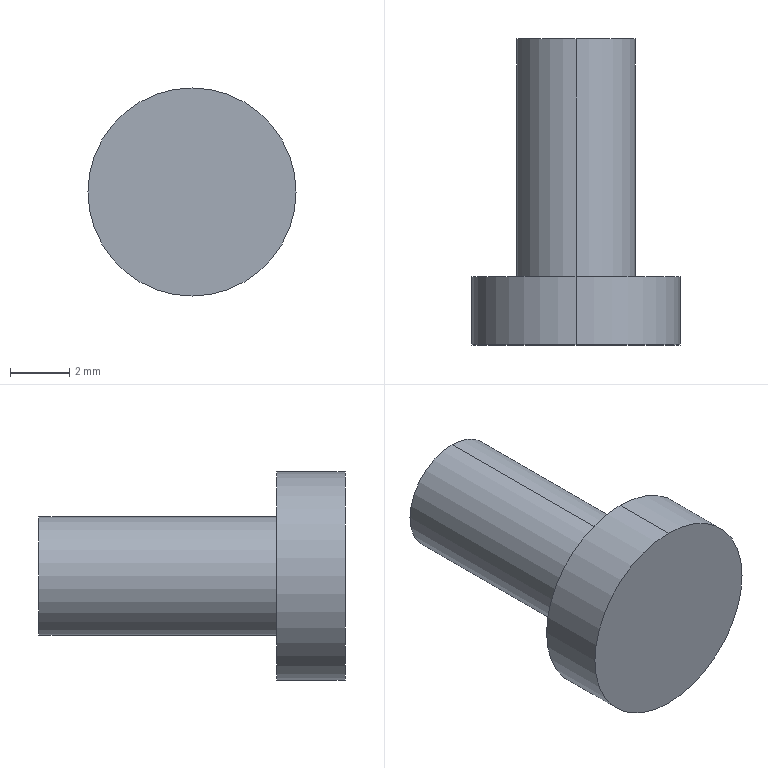Part | SolidWorks | features Extrusion 1, ICE 1 | 1 solid | 7 faces | box 7 x 10.3 x 7 mm | volume 189.045 mm3 | cylinder 4 | plane 3 | commonest cylinder face diameters 4 x2 7 x2
STEP:
#1=CARTESIAN_POINT('',(0.,-2.3,-3.5));
#2=VERTEX_POINT('',#1);
#3=CARTESIAN_POINT('',(0.,-2.3,3.5));
#4=VERTEX_POINT('',#3);
#5=CARTESIAN_POINT('',(0.,-2.3,0.));
#6=DIRECTION('',(0.,-1.,0.));
#7=DIRECTION('',(0.,0.,-1.));
#8=AXIS2_PLACEMENT_3D('',#5,#6,#7);
#9=CIRCLE('',#8,3.5);
#10=EDGE_CURVE('',#2,#4,#9,.T.);
#11=ORIENTED_EDGE('',*,*,#10,.F.);
#12=CARTESIAN_POINT('',(0.,0.,-3.5));
#13=VERTEX_POINT('',#12);
#14=CARTESIAN_POINT('',(0.,-2.3,-3.5));
#15=DIRECTION('',(0.,1.,0.));
#16=VECTOR('',#15,1000.);
#17=LINE('',#14,#16);
#18=EDGE_CURVE('',#2,#13,#17,.T.);
#19=ORIENTED_EDGE('',*,*,#18,.T.);
#20=CARTESIAN_POINT('',(0.,0.,3.5));
#21=VERTEX_POINT('',#20);
#22=CARTESIAN_POINT('',(0.,0.,0.));
#23=DIRECTION('',(0.,-1.,0.));
#24=DIRECTION('',(0.,0.,-1.));
#25=AXIS2_PLACEMENT_3D('',#22,#23,#24);
#26=CIRCLE('',#25,3.5);
#27=EDGE_CURVE('',#13,#21,#26,.T.);
#28=ORIENTED_EDGE('',*,*,#27,.T.);
#29=CARTESIAN_POINT('',(0.,-2.3,3.5));
#30=DIRECTION('',(0.,1.,0.));
#31=VECTOR('',#30,1000.);
#32=LINE('',#29,#31);
#33=EDGE_CURVE('',#4,#21,#32,.T.);
#34=ORIENTED_EDGE('',*,*,#33,.F.);
#35=EDGE_LOOP('',(#11,#19,#28,#34));
#36=FACE_OUTER_BOUND('',#35,.T.);
#37=CARTESIAN_POINT('',(0.,-2.3,0.));
#38=DIRECTION('',(0.,1.,0.));
#39=DIRECTION('',(0.,0.,1.));
#40=AXIS2_PLACEMENT_3D('',#37,#38,#39);
#41=CYLINDRICAL_SURFACE('',#40,3.5);
#42=ADVANCED_FACE('',(#36),#41,.T.);
#43=CARTESIAN_POINT('',(0.,8.,2.));
#44=VERTEX_POINT('',#43);
#45=CARTESIAN_POINT('',(0.,8.,-2.));
#46=VERTEX_POINT('',#45);
#47=CARTESIAN_POINT('',(0.,8.,0.));
#48=DIRECTION('',(0.,1.,0.));
#49=DIRECTION('',(0.,0.,1.));
#50=AXIS2_PLACEMENT_3D('',#47,#48,#49);
#51=CIRCLE('',#50,2.);
#52=EDGE_CURVE('',#44,#46,#51,.T.);
#53=ORIENTED_EDGE('',*,*,#52,.F.);
#54=CARTESIAN_POINT('',(0.,0.,2.));
#55=VERTEX_POINT('',#54);
#56=CARTESIAN_POINT('',(0.,8.,2.));
#57=DIRECTION('',(0.,-1.,0.));
#58=VECTOR('',#57,1000.);
#59=LINE('',#56,#58);
#60=EDGE_CURVE('',#44,#55,#59,.T.);
#61=ORIENTED_EDGE('',*,*,#60,.T.);
#62=CARTESIAN_POINT('',(0.,0.,-2.));
#63=VERTEX_POINT('',#62);
#64=CARTESIAN_POINT('',(0.,0.,0.));
#65=DIRECTION('',(0.,1.,0.));
#66=DIRECTION('',(0.,0.,1.));
#67=AXIS2_PLACEMENT_3D('',#64,#65,#66);
#68=CIRCLE('',#67,2.);
#69=EDGE_CURVE('',#55,#63,#68,.T.);
#70=ORIENTED_EDGE('',*,*,#69,.T.);
#71=CARTESIAN_POINT('',(0.,8.,-2.));
#72=DIRECTION('',(0.,-1.,0.));
#73=VECTOR('',#72,1000.);
#74=LINE('',#71,#73);
#75=EDGE_CURVE('',#46,#63,#74,.T.);
#76=ORIENTED_EDGE('',*,*,#75,.F.);
#77=EDGE_LOOP('',(#53,#61,#70,#76));
#78=FACE_OUTER_BOUND('',#77,.T.);
#79=CARTESIAN_POINT('',(0.,8.,0.));
#80=DIRECTION('',(0.,-1.,0.));
#81=DIRECTION('',(0.,0.,-1.));
#82=AXIS2_PLACEMENT_3D('',#79,#80,#81);
#83=CYLINDRICAL_SURFACE('',#82,2.);
#84=ADVANCED_FACE('',(#78),#83,.T.);
#85=ORIENTED_EDGE('',*,*,#60,.F.);
#86=CARTESIAN_POINT('',(0.,8.,0.));
#87=DIRECTION('',(0.,1.,0.));
#88=DIRECTION('',(0.,0.,1.));
#89=AXIS2_PLACEMENT_3D('',#86,#87,#88);
#90=CIRCLE('',#89,2.);
#91=EDGE_CURVE('',#46,#44,#90,.T.);
#92=ORIENTED_EDGE('',*,*,#91,.F.);
#93=ORIENTED_EDGE('',*,*,#75,.T.);
#94=CARTESIAN_POINT('',(0.,0.,0.));
#95=DIRECTION('',(0.,1.,0.));
#96=DIRECTION('',(0.,0.,1.));
#97=AXIS2_PLACEMENT_3D('',#94,#95,#96);
#98=CIRCLE('',#97,2.);
#99=EDGE_CURVE('',#63,#55,#98,.T.);
#100=ORIENTED_EDGE('',*,*,#99,.T.);
#101=EDGE_LOOP('',(#85,#92,#93,#100));
#102=FACE_OUTER_BOUND('',#101,.T.);
#103=CARTESIAN_POINT('',(0.,8.,0.));
#104=DIRECTION('',(0.,-1.,0.));
#105=DIRECTION('',(0.,0.,-1.));
#106=AXIS2_PLACEMENT_3D('',#103,#104,#105);
#107=CYLINDRICAL_SURFACE('',#106,2.);
#108=ADVANCED_FACE('',(#102),#107,.T.);
#109=ORIENTED_EDGE('',*,*,#91,.T.);
#110=ORIENTED_EDGE('',*,*,#52,.T.);
#111=EDGE_LOOP('',(#109,#110));
#112=FACE_OUTER_BOUND('',#111,.T.);
#113=CARTESIAN_POINT('',(0.,8.,0.));
#114=DIRECTION('',(0.,1.,0.));
#115=DIRECTION('',(0.,0.,1.));
#116=AXIS2_PLACEMENT_3D('',#113,#114,#115);
#117=PLANE('',#116);
#118=ADVANCED_FACE('',(#112),#117,.T.);
#119=ORIENTED_EDGE('',*,*,#18,.F.);
#120=CARTESIAN_POINT('',(0.,-2.3,0.));
#121=DIRECTION('',(0.,-1.,0.));
#122=DIRECTION('',(0.,0.,-1.));
#123=AXIS2_PLACEMENT_3D('',#120,#121,#122);
#124=CIRCLE('',#123,3.5);
#125=EDGE_CURVE('',#4,#2,#124,.T.);
#126=ORIENTED_EDGE('',*,*,#125,.F.);
#127=ORIENTED_EDGE('',*,*,#33,.T.);
#128=CARTESIAN_POINT('',(0.,0.,0.));
#129=DIRECTION('',(0.,-1.,0.));
#130=DIRECTION('',(0.,0.,-1.));
#131=AXIS2_PLACEMENT_3D('',#128,#129,#130);
#132=CIRCLE('',#131,3.5);
#133=EDGE_CURVE('',#21,#13,#132,.T.);
#134=ORIENTED_EDGE('',*,*,#133,.T.);
#135=EDGE_LOOP('',(#119,#126,#127,#134));
#136=FACE_OUTER_BOUND('',#135,.T.);
#137=CARTESIAN_POINT('',(0.,-2.3,0.));
#138=DIRECTION('',(0.,1.,0.));
#139=DIRECTION('',(0.,0.,1.));
#140=AXIS2_PLACEMENT_3D('',#137,#138,#139);
#141=CYLINDRICAL_SURFACE('',#140,3.5);
#142=ADVANCED_FACE('',(#136),#141,.T.);
#143=ORIENTED_EDGE('',*,*,#125,.T.);
#144=ORIENTED_EDGE('',*,*,#10,.T.);
#145=EDGE_LOOP('',(#143,#144));
#146=FACE_OUTER_BOUND('',#145,.T.);
#147=CARTESIAN_POINT('',(0.,-2.3,0.));
#148=DIRECTION('',(0.,-1.,0.));
#149=DIRECTION('',(0.,0.,-1.));
#150=AXIS2_PLACEMENT_3D('',#147,#148,#149);
#151=PLANE('',#150);
#152=ADVANCED_FACE('',(#146),#151,.T.);
#153=ORIENTED_EDGE('',*,*,#99,.F.);
#154=ORIENTED_EDGE('',*,*,#69,.F.);
#155=EDGE_LOOP('',(#153,#154));
#156=FACE_BOUND('',#155,.T.);
#157=ORIENTED_EDGE('',*,*,#133,.F.);
#158=ORIENTED_EDGE('',*,*,#27,.F.);
#159=EDGE_LOOP('',(#157,#158));
#160=FACE_OUTER_BOUND('',#159,.T.);
#161=CARTESIAN_POINT('',(0.,0.,0.));
#162=DIRECTION('',(0.,-1.,0.));
#163=DIRECTION('',(0.,0.,-1.));
#164=AXIS2_PLACEMENT_3D('',#161,#162,#163);
#165=PLANE('',#164);
#166=ADVANCED_FACE('',(#156,#160),#165,.F.);
#167=CLOSED_SHELL('',(#42,#84,#108,#118,#142,#152,#166));
#168=MANIFOLD_SOLID_BREP('',#167);
#169=CARTESIAN_POINT('',(0.,0.,0.));
#170=DIRECTION('',(0.,0.,1.));
#171=DIRECTION('',(1.,0.,0.));
#172=AXIS2_PLACEMENT_3D('',#169,#170,#171);
#173=(LENGTH_UNIT()NAMED_UNIT(*)SI_UNIT(.MILLI.,.METRE.));
#174=UNCERTAINTY_MEASURE_WITH_UNIT(LENGTH_MEASURE(0.00001),#173,'','');
#175=(NAMED_UNIT(*)PLANE_ANGLE_UNIT()SI_UNIT($,.RADIAN.));
#176=(NAMED_UNIT(*)SI_UNIT($,.STERADIAN.)SOLID_ANGLE_UNIT());
#177=(GEOMETRIC_REPRESENTATION_CONTEXT(3)GLOBAL_UNCERTAINTY_ASSIGNED_CONTEXT((#174))GLOBAL_UNIT_ASSIGNED_CONTEXT((#173,#175,#176))REPRESENTATION_CONTEXT('',''));
#178=ADVANCED_BREP_SHAPE_REPRESENTATION('',(#168,#172),#177);